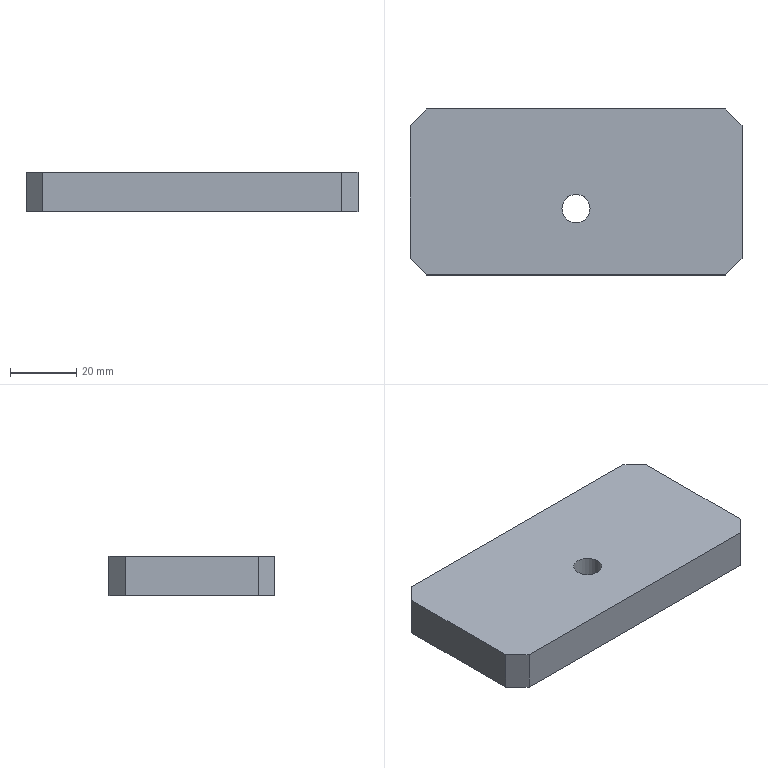Part | NX | features BREP 1 | 1 solid | 11 faces | box 100 x 50 x 12 mm | volume 58719 mm3 | plane 10 | cylinder 1 | commonest cylinder face diameters 8.5 x1
STEP:
#1=CARTESIAN_POINT('',(50.,-20.,12.));
#2=VERTEX_POINT('',#1);
#3=CARTESIAN_POINT('',(50.,20.,12.));
#4=VERTEX_POINT('',#3);
#5=CARTESIAN_POINT('',(50.,25.,12.));
#6=DIRECTION('',(0.,1.,0.));
#7=VECTOR('',#6,1000.);
#8=LINE('',#5,#7);
#9=EDGE_CURVE('',#2,#4,#8,.T.);
#10=ORIENTED_EDGE('',*,*,#9,.F.);
#11=CARTESIAN_POINT('',(50.,-20.,0.));
#12=VERTEX_POINT('',#11);
#13=CARTESIAN_POINT('',(50.,-20.,15.));
#14=DIRECTION('',(0.,0.,-1.));
#15=VECTOR('',#14,1000.);
#16=LINE('',#13,#15);
#17=EDGE_CURVE('',#2,#12,#16,.T.);
#18=ORIENTED_EDGE('',*,*,#17,.T.);
#19=CARTESIAN_POINT('',(50.,20.,0.));
#20=VERTEX_POINT('',#19);
#21=CARTESIAN_POINT('',(50.,25.,0.));
#22=DIRECTION('',(0.,1.,0.));
#23=VECTOR('',#22,1000.);
#24=LINE('',#21,#23);
#25=EDGE_CURVE('',#12,#20,#24,.T.);
#26=ORIENTED_EDGE('',*,*,#25,.T.);
#27=CARTESIAN_POINT('',(50.,20.,15.));
#28=DIRECTION('',(0.,0.,1.));
#29=VECTOR('',#28,1000.);
#30=LINE('',#27,#29);
#31=EDGE_CURVE('',#20,#4,#30,.T.);
#32=ORIENTED_EDGE('',*,*,#31,.T.);
#33=EDGE_LOOP('',(#10,#18,#26,#32));
#34=FACE_BOUND('',#33,.T.);
#35=CARTESIAN_POINT('',(50.,25.,15.));
#36=DIRECTION('',(-1.,0.,0.));
#37=DIRECTION('',(0.,0.,-1.));
#38=AXIS2_PLACEMENT_3D('',#35,#36,#37);
#39=PLANE('',#38);
#40=ADVANCED_FACE('',(#34),#39,.F.);
#41=CARTESIAN_POINT('',(45.,25.,12.));
#42=VERTEX_POINT('',#41);
#43=CARTESIAN_POINT('',(-45.,25.,12.));
#44=VERTEX_POINT('',#43);
#45=CARTESIAN_POINT('',(-50.,25.,12.));
#46=DIRECTION('',(-1.,0.,0.));
#47=VECTOR('',#46,1000.);
#48=LINE('',#45,#47);
#49=EDGE_CURVE('',#42,#44,#48,.T.);
#50=ORIENTED_EDGE('',*,*,#49,.F.);
#51=CARTESIAN_POINT('',(45.,25.,0.));
#52=VERTEX_POINT('',#51);
#53=CARTESIAN_POINT('',(45.,25.,15.));
#54=DIRECTION('',(0.,0.,-1.));
#55=VECTOR('',#54,1000.);
#56=LINE('',#53,#55);
#57=EDGE_CURVE('',#42,#52,#56,.T.);
#58=ORIENTED_EDGE('',*,*,#57,.T.);
#59=CARTESIAN_POINT('',(-45.,25.,0.));
#60=VERTEX_POINT('',#59);
#61=CARTESIAN_POINT('',(-50.,25.,0.));
#62=DIRECTION('',(-1.,0.,0.));
#63=VECTOR('',#62,1000.);
#64=LINE('',#61,#63);
#65=EDGE_CURVE('',#52,#60,#64,.T.);
#66=ORIENTED_EDGE('',*,*,#65,.T.);
#67=CARTESIAN_POINT('',(-45.,25.,15.));
#68=DIRECTION('',(0.,0.,1.));
#69=VECTOR('',#68,1000.);
#70=LINE('',#67,#69);
#71=EDGE_CURVE('',#60,#44,#70,.T.);
#72=ORIENTED_EDGE('',*,*,#71,.T.);
#73=EDGE_LOOP('',(#50,#58,#66,#72));
#74=FACE_BOUND('',#73,.T.);
#75=CARTESIAN_POINT('',(-50.,25.,15.));
#76=DIRECTION('',(0.,-1.,0.));
#77=DIRECTION('',(0.,0.,1.));
#78=AXIS2_PLACEMENT_3D('',#75,#76,#77);
#79=PLANE('',#78);
#80=ADVANCED_FACE('',(#74),#79,.F.);
#81=CARTESIAN_POINT('',(-50.,20.,12.));
#82=VERTEX_POINT('',#81);
#83=CARTESIAN_POINT('',(-50.,-20.,12.));
#84=VERTEX_POINT('',#83);
#85=CARTESIAN_POINT('',(-50.,25.,12.));
#86=DIRECTION('',(0.,-1.,0.));
#87=VECTOR('',#86,1000.);
#88=LINE('',#85,#87);
#89=EDGE_CURVE('',#82,#84,#88,.T.);
#90=ORIENTED_EDGE('',*,*,#89,.F.);
#91=CARTESIAN_POINT('',(-50.,20.,0.));
#92=VERTEX_POINT('',#91);
#93=CARTESIAN_POINT('',(-50.,20.,15.));
#94=DIRECTION('',(0.,0.,-1.));
#95=VECTOR('',#94,1000.);
#96=LINE('',#93,#95);
#97=EDGE_CURVE('',#82,#92,#96,.T.);
#98=ORIENTED_EDGE('',*,*,#97,.T.);
#99=CARTESIAN_POINT('',(-50.,-20.,0.));
#100=VERTEX_POINT('',#99);
#101=CARTESIAN_POINT('',(-50.,25.,0.));
#102=DIRECTION('',(0.,-1.,0.));
#103=VECTOR('',#102,1000.);
#104=LINE('',#101,#103);
#105=EDGE_CURVE('',#92,#100,#104,.T.);
#106=ORIENTED_EDGE('',*,*,#105,.T.);
#107=CARTESIAN_POINT('',(-50.,-20.,15.));
#108=DIRECTION('',(0.,0.,1.));
#109=VECTOR('',#108,1000.);
#110=LINE('',#107,#109);
#111=EDGE_CURVE('',#100,#84,#110,.T.);
#112=ORIENTED_EDGE('',*,*,#111,.T.);
#113=EDGE_LOOP('',(#90,#98,#106,#112));
#114=FACE_BOUND('',#113,.T.);
#115=CARTESIAN_POINT('',(-50.,25.,15.));
#116=DIRECTION('',(1.,0.,0.));
#117=DIRECTION('',(0.,0.,1.));
#118=AXIS2_PLACEMENT_3D('',#115,#116,#117);
#119=PLANE('',#118);
#120=ADVANCED_FACE('',(#114),#119,.F.);
#121=CARTESIAN_POINT('',(45.,-25.,12.));
#122=VERTEX_POINT('',#121);
#123=CARTESIAN_POINT('',(-45.,-25.,12.));
#124=VERTEX_POINT('',#123);
#125=CARTESIAN_POINT('',(950.,-25.,12.));
#126=DIRECTION('',(-1.,0.,0.));
#127=VECTOR('',#126,1000.);
#128=LINE('',#125,#127);
#129=EDGE_CURVE('',#122,#124,#128,.T.);
#130=ORIENTED_EDGE('',*,*,#129,.T.);
#131=CARTESIAN_POINT('',(-45.,-25.,0.));
#132=VERTEX_POINT('',#131);
#133=CARTESIAN_POINT('',(-45.,-25.,15.));
#134=DIRECTION('',(0.,0.,-1.));
#135=VECTOR('',#134,1000.);
#136=LINE('',#133,#135);
#137=EDGE_CURVE('',#124,#132,#136,.T.);
#138=ORIENTED_EDGE('',*,*,#137,.T.);
#139=CARTESIAN_POINT('',(45.,-25.,0.));
#140=VERTEX_POINT('',#139);
#141=CARTESIAN_POINT('',(-50.,-25.,0.));
#142=DIRECTION('',(1.,0.,0.));
#143=VECTOR('',#142,1000.);
#144=LINE('',#141,#143);
#145=EDGE_CURVE('',#132,#140,#144,.T.);
#146=ORIENTED_EDGE('',*,*,#145,.T.);
#147=CARTESIAN_POINT('',(45.,-25.,15.));
#148=DIRECTION('',(0.,0.,1.));
#149=VECTOR('',#148,1000.);
#150=LINE('',#147,#149);
#151=EDGE_CURVE('',#140,#122,#150,.T.);
#152=ORIENTED_EDGE('',*,*,#151,.T.);
#153=EDGE_LOOP('',(#130,#138,#146,#152));
#154=FACE_BOUND('',#153,.T.);
#155=CARTESIAN_POINT('',(-50.,-25.,15.));
#156=DIRECTION('',(0.,1.,0.));
#157=DIRECTION('',(0.,0.,-1.));
#158=AXIS2_PLACEMENT_3D('',#155,#156,#157);
#159=PLANE('',#158);
#160=ADVANCED_FACE('',(#154),#159,.F.);
#161=ORIENTED_EDGE('',*,*,#137,.F.);
#162=CARTESIAN_POINT('',(-45.,-25.,12.));
#163=DIRECTION('',(-0.7071,0.7071,0.));
#164=VECTOR('',#163,1000.);
#165=LINE('',#162,#164);
#166=EDGE_CURVE('',#124,#84,#165,.T.);
#167=ORIENTED_EDGE('',*,*,#166,.T.);
#168=ORIENTED_EDGE('',*,*,#111,.F.);
#169=CARTESIAN_POINT('',(-45.,-25.,0.));
#170=DIRECTION('',(-0.7071,0.7071,0.));
#171=VECTOR('',#170,1000.);
#172=LINE('',#169,#171);
#173=EDGE_CURVE('',#132,#100,#172,.T.);
#174=ORIENTED_EDGE('',*,*,#173,.F.);
#175=EDGE_LOOP('',(#161,#167,#168,#174));
#176=FACE_BOUND('',#175,.T.);
#177=CARTESIAN_POINT('',(-45.,-25.,15.));
#178=DIRECTION('',(0.7071,0.7071,0.));
#179=DIRECTION('',(0.,0.,1.));
#180=AXIS2_PLACEMENT_3D('',#177,#178,#179);
#181=PLANE('',#180);
#182=ADVANCED_FACE('',(#176),#181,.F.);
#183=ORIENTED_EDGE('',*,*,#97,.F.);
#184=CARTESIAN_POINT('',(-50.,20.,12.));
#185=DIRECTION('',(0.7071,0.7071,0.));
#186=VECTOR('',#185,1000.);
#187=LINE('',#184,#186);
#188=EDGE_CURVE('',#82,#44,#187,.T.);
#189=ORIENTED_EDGE('',*,*,#188,.T.);
#190=ORIENTED_EDGE('',*,*,#71,.F.);
#191=CARTESIAN_POINT('',(-50.,20.,0.));
#192=DIRECTION('',(0.7071,0.7071,0.));
#193=VECTOR('',#192,1000.);
#194=LINE('',#191,#193);
#195=EDGE_CURVE('',#92,#60,#194,.T.);
#196=ORIENTED_EDGE('',*,*,#195,.F.);
#197=EDGE_LOOP('',(#183,#189,#190,#196));
#198=FACE_BOUND('',#197,.T.);
#199=CARTESIAN_POINT('',(-50.,20.,15.));
#200=DIRECTION('',(0.7071,-0.7071,0.));
#201=DIRECTION('',(0.,0.,1.));
#202=AXIS2_PLACEMENT_3D('',#199,#200,#201);
#203=PLANE('',#202);
#204=ADVANCED_FACE('',(#198),#203,.F.);
#205=ORIENTED_EDGE('',*,*,#17,.F.);
#206=CARTESIAN_POINT('',(50.,-20.,12.));
#207=DIRECTION('',(-0.7071,-0.7071,0.));
#208=VECTOR('',#207,1000.);
#209=LINE('',#206,#208);
#210=EDGE_CURVE('',#2,#122,#209,.T.);
#211=ORIENTED_EDGE('',*,*,#210,.T.);
#212=ORIENTED_EDGE('',*,*,#151,.F.);
#213=CARTESIAN_POINT('',(50.,-20.,0.));
#214=DIRECTION('',(-0.7071,-0.7071,0.));
#215=VECTOR('',#214,1000.);
#216=LINE('',#213,#215);
#217=EDGE_CURVE('',#12,#140,#216,.T.);
#218=ORIENTED_EDGE('',*,*,#217,.F.);
#219=EDGE_LOOP('',(#205,#211,#212,#218));
#220=FACE_BOUND('',#219,.T.);
#221=CARTESIAN_POINT('',(50.,-20.,15.));
#222=DIRECTION('',(-0.7071,0.7071,0.));
#223=DIRECTION('',(0.,0.,1.));
#224=AXIS2_PLACEMENT_3D('',#221,#222,#223);
#225=PLANE('',#224);
#226=ADVANCED_FACE('',(#220),#225,.F.);
#227=ORIENTED_EDGE('',*,*,#57,.F.);
#228=CARTESIAN_POINT('',(45.,25.,12.));
#229=DIRECTION('',(0.7071,-0.7071,0.));
#230=VECTOR('',#229,1000.);
#231=LINE('',#228,#230);
#232=EDGE_CURVE('',#42,#4,#231,.T.);
#233=ORIENTED_EDGE('',*,*,#232,.T.);
#234=ORIENTED_EDGE('',*,*,#31,.F.);
#235=CARTESIAN_POINT('',(45.,25.,0.));
#236=DIRECTION('',(0.7071,-0.7071,0.));
#237=VECTOR('',#236,1000.);
#238=LINE('',#235,#237);
#239=EDGE_CURVE('',#52,#20,#238,.T.);
#240=ORIENTED_EDGE('',*,*,#239,.F.);
#241=EDGE_LOOP('',(#227,#233,#234,#240));
#242=FACE_BOUND('',#241,.T.);
#243=CARTESIAN_POINT('',(45.,25.,15.));
#244=DIRECTION('',(-0.7071,-0.7071,0.));
#245=DIRECTION('',(0.,0.,1.));
#246=AXIS2_PLACEMENT_3D('',#243,#244,#245);
#247=PLANE('',#246);
#248=ADVANCED_FACE('',(#242),#247,.F.);
#249=CARTESIAN_POINT('',(4.25,-5.,0.));
#250=VERTEX_POINT('',#249);
#251=CARTESIAN_POINT('',(0.,-5.,0.));
#252=DIRECTION('',(0.,0.,1.));
#253=DIRECTION('',(1.,0.,0.));
#254=AXIS2_PLACEMENT_3D('',#251,#252,#253);
#255=CIRCLE('',#254,4.25);
#256=EDGE_CURVE('',#250,#250,#255,.T.);
#257=ORIENTED_EDGE('',*,*,#256,.T.);
#258=EDGE_LOOP('',(#257));
#259=FACE_BOUND('',#258,.T.);
#260=ORIENTED_EDGE('',*,*,#145,.F.);
#261=ORIENTED_EDGE('',*,*,#173,.T.);
#262=ORIENTED_EDGE('',*,*,#105,.F.);
#263=ORIENTED_EDGE('',*,*,#195,.T.);
#264=ORIENTED_EDGE('',*,*,#65,.F.);
#265=ORIENTED_EDGE('',*,*,#239,.T.);
#266=ORIENTED_EDGE('',*,*,#25,.F.);
#267=ORIENTED_EDGE('',*,*,#217,.T.);
#268=EDGE_LOOP('',(#260,#261,#262,#263,#264,#265,#266,#267));
#269=FACE_BOUND('',#268,.T.);
#270=CARTESIAN_POINT('',(0.,0.,0.));
#271=DIRECTION('',(0.,0.,1.));
#272=DIRECTION('',(-1.,0.,0.));
#273=AXIS2_PLACEMENT_3D('',#270,#271,#272);
#274=PLANE('',#273);
#275=ADVANCED_FACE('',(#259,#269),#274,.F.);
#276=CARTESIAN_POINT('',(-4.25,-5.,12.));
#277=VERTEX_POINT('',#276);
#278=CARTESIAN_POINT('',(0.,-5.,12.));
#279=DIRECTION('',(0.,0.,1.));
#280=DIRECTION('',(-1.,0.,0.));
#281=AXIS2_PLACEMENT_3D('',#278,#279,#280);
#282=CIRCLE('',#281,4.25);
#283=EDGE_CURVE('',#277,#277,#282,.T.);
#284=ORIENTED_EDGE('',*,*,#283,.F.);
#285=EDGE_LOOP('',(#284));
#286=FACE_BOUND('',#285,.T.);
#287=ORIENTED_EDGE('',*,*,#129,.F.);
#288=ORIENTED_EDGE('',*,*,#210,.F.);
#289=ORIENTED_EDGE('',*,*,#9,.T.);
#290=ORIENTED_EDGE('',*,*,#232,.F.);
#291=ORIENTED_EDGE('',*,*,#49,.T.);
#292=ORIENTED_EDGE('',*,*,#188,.F.);
#293=ORIENTED_EDGE('',*,*,#89,.T.);
#294=ORIENTED_EDGE('',*,*,#166,.F.);
#295=EDGE_LOOP('',(#287,#288,#289,#290,#291,#292,#293,#294));
#296=FACE_BOUND('',#295,.T.);
#297=CARTESIAN_POINT('',(0.,325.,12.));
#298=DIRECTION('',(0.,0.,1.));
#299=DIRECTION('',(1.,0.,0.));
#300=AXIS2_PLACEMENT_3D('',#297,#298,#299);
#301=PLANE('',#300);
#302=ADVANCED_FACE('',(#286,#296),#301,.T.);
#303=ORIENTED_EDGE('',*,*,#283,.T.);
#304=EDGE_LOOP('',(#303));
#305=FACE_BOUND('',#304,.T.);
#306=ORIENTED_EDGE('',*,*,#256,.F.);
#307=EDGE_LOOP('',(#306));
#308=FACE_BOUND('',#307,.T.);
#309=CARTESIAN_POINT('',(0.,-5.,12.));
#310=DIRECTION('',(0.,0.,1.));
#311=DIRECTION('',(1.,0.,0.));
#312=AXIS2_PLACEMENT_3D('',#309,#310,#311);
#313=CYLINDRICAL_SURFACE('',#312,4.25);
#314=ADVANCED_FACE('',(#305,#308),#313,.F.);
#315=CLOSED_SHELL('',(#40,#80,#120,#160,#182,#204,#226,#248,#275,#302,#314));
#316=MANIFOLD_SOLID_BREP('',#315);
#317=(LENGTH_UNIT()NAMED_UNIT(*)SI_UNIT(.MILLI.,.METRE.));
#318=UNCERTAINTY_MEASURE_WITH_UNIT(LENGTH_MEASURE(0.00001),#317,'','');
#319=(NAMED_UNIT(*)PLANE_ANGLE_UNIT()SI_UNIT($,.RADIAN.));
#320=(NAMED_UNIT(*)SI_UNIT($,.STERADIAN.)SOLID_ANGLE_UNIT());
#321=(GEOMETRIC_REPRESENTATION_CONTEXT(3)GLOBAL_UNCERTAINTY_ASSIGNED_CONTEXT((#318))GLOBAL_UNIT_ASSIGNED_CONTEXT((#317,#319,#320))REPRESENTATION_CONTEXT('',''));
#322=ADVANCED_BREP_SHAPE_REPRESENTATION('',(#316),#321);